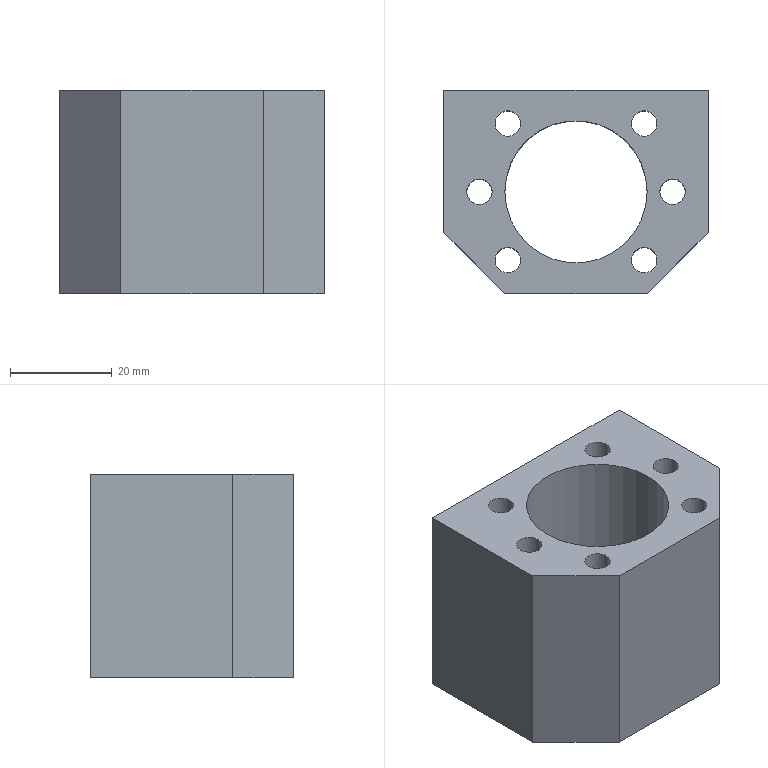Part | SolidWorks | features BaseBody 1 | 1 solid | 34 faces | box 52 x 40 x 40 mm | volume 47312 mm3 | cylinder 22 | plane 12 | commonest cylinder face diameters 5 x20 28 x2
STEP:
#1=CARTESIAN_POINT('',(-17.5,10.,8.));
#2=VERTEX_POINT('',#1);
#3=CARTESIAN_POINT('',(-22.5,10.,8.));
#4=VERTEX_POINT('',#3);
#5=CARTESIAN_POINT('',(-20.,10.,8.));
#6=DIRECTION('',(0.,1.,0.));
#7=DIRECTION('',(-1.,0.,0.));
#8=AXIS2_PLACEMENT_3D('',#5,#6,#7);
#9=CIRCLE('',#8,2.5);
#10=EDGE_CURVE('',#2,#4,#9,.T.);
#11=ORIENTED_EDGE('',*,*,#10,.F.);
#12=CARTESIAN_POINT('',(-17.5,20.,8.));
#13=VERTEX_POINT('',#12);
#14=CARTESIAN_POINT('',(-17.5,10.,8.));
#15=DIRECTION('',(0.,1.,0.));
#16=VECTOR('',#15,1000.);
#17=LINE('',#14,#16);
#18=EDGE_CURVE('',#2,#13,#17,.T.);
#19=ORIENTED_EDGE('',*,*,#18,.T.);
#20=CARTESIAN_POINT('',(-22.5,20.,8.));
#21=VERTEX_POINT('',#20);
#22=CARTESIAN_POINT('',(-20.,20.,8.));
#23=DIRECTION('',(0.,1.,0.));
#24=DIRECTION('',(-1.,0.,0.));
#25=AXIS2_PLACEMENT_3D('',#22,#23,#24);
#26=CIRCLE('',#25,2.5);
#27=EDGE_CURVE('',#13,#21,#26,.T.);
#28=ORIENTED_EDGE('',*,*,#27,.T.);
#29=CARTESIAN_POINT('',(-22.5,10.,8.));
#30=DIRECTION('',(0.,1.,0.));
#31=VECTOR('',#30,1000.);
#32=LINE('',#29,#31);
#33=EDGE_CURVE('',#4,#21,#32,.T.);
#34=ORIENTED_EDGE('',*,*,#33,.F.);
#35=EDGE_LOOP('',(#11,#19,#28,#34));
#36=FACE_OUTER_BOUND('',#35,.T.);
#37=CARTESIAN_POINT('',(-20.,10.,8.));
#38=DIRECTION('',(0.,1.,0.));
#39=DIRECTION('',(-1.,0.,0.));
#40=AXIS2_PLACEMENT_3D('',#37,#38,#39);
#41=CYLINDRICAL_SURFACE('',#40,2.5);
#42=ADVANCED_FACE('',(#36),#41,.F.);
#43=CARTESIAN_POINT('',(-17.5,10.,32.));
#44=VERTEX_POINT('',#43);
#45=CARTESIAN_POINT('',(-22.5,10.,32.));
#46=VERTEX_POINT('',#45);
#47=CARTESIAN_POINT('',(-20.,10.,32.));
#48=DIRECTION('',(0.,1.,0.));
#49=DIRECTION('',(-1.,0.,0.));
#50=AXIS2_PLACEMENT_3D('',#47,#48,#49);
#51=CIRCLE('',#50,2.5);
#52=EDGE_CURVE('',#44,#46,#51,.T.);
#53=ORIENTED_EDGE('',*,*,#52,.F.);
#54=CARTESIAN_POINT('',(-17.5,20.,32.));
#55=VERTEX_POINT('',#54);
#56=CARTESIAN_POINT('',(-17.5,10.,32.));
#57=DIRECTION('',(0.,1.,0.));
#58=VECTOR('',#57,1000.);
#59=LINE('',#56,#58);
#60=EDGE_CURVE('',#44,#55,#59,.T.);
#61=ORIENTED_EDGE('',*,*,#60,.T.);
#62=CARTESIAN_POINT('',(-22.5,20.,32.));
#63=VERTEX_POINT('',#62);
#64=CARTESIAN_POINT('',(-20.,20.,32.));
#65=DIRECTION('',(0.,1.,0.));
#66=DIRECTION('',(-1.,0.,0.));
#67=AXIS2_PLACEMENT_3D('',#64,#65,#66);
#68=CIRCLE('',#67,2.5);
#69=EDGE_CURVE('',#55,#63,#68,.T.);
#70=ORIENTED_EDGE('',*,*,#69,.T.);
#71=CARTESIAN_POINT('',(-22.5,10.,32.));
#72=DIRECTION('',(0.,1.,0.));
#73=VECTOR('',#72,1000.);
#74=LINE('',#71,#73);
#75=EDGE_CURVE('',#46,#63,#74,.T.);
#76=ORIENTED_EDGE('',*,*,#75,.F.);
#77=EDGE_LOOP('',(#53,#61,#70,#76));
#78=FACE_OUTER_BOUND('',#77,.T.);
#79=CARTESIAN_POINT('',(-20.,10.,32.));
#80=DIRECTION('',(0.,1.,0.));
#81=DIRECTION('',(-1.,0.,0.));
#82=AXIS2_PLACEMENT_3D('',#79,#80,#81);
#83=CYLINDRICAL_SURFACE('',#82,2.5);
#84=ADVANCED_FACE('',(#78),#83,.F.);
#85=CARTESIAN_POINT('',(22.5,10.,32.));
#86=VERTEX_POINT('',#85);
#87=CARTESIAN_POINT('',(17.5,10.,32.));
#88=VERTEX_POINT('',#87);
#89=CARTESIAN_POINT('',(20.,10.,32.));
#90=DIRECTION('',(0.,1.,0.));
#91=DIRECTION('',(-1.,0.,0.));
#92=AXIS2_PLACEMENT_3D('',#89,#90,#91);
#93=CIRCLE('',#92,2.5);
#94=EDGE_CURVE('',#86,#88,#93,.T.);
#95=ORIENTED_EDGE('',*,*,#94,.F.);
#96=CARTESIAN_POINT('',(22.5,20.,32.));
#97=VERTEX_POINT('',#96);
#98=CARTESIAN_POINT('',(22.5,10.,32.));
#99=DIRECTION('',(0.,1.,0.));
#100=VECTOR('',#99,1000.);
#101=LINE('',#98,#100);
#102=EDGE_CURVE('',#86,#97,#101,.T.);
#103=ORIENTED_EDGE('',*,*,#102,.T.);
#104=CARTESIAN_POINT('',(17.5,20.,32.));
#105=VERTEX_POINT('',#104);
#106=CARTESIAN_POINT('',(20.,20.,32.));
#107=DIRECTION('',(0.,1.,0.));
#108=DIRECTION('',(-1.,0.,0.));
#109=AXIS2_PLACEMENT_3D('',#106,#107,#108);
#110=CIRCLE('',#109,2.5);
#111=EDGE_CURVE('',#97,#105,#110,.T.);
#112=ORIENTED_EDGE('',*,*,#111,.T.);
#113=CARTESIAN_POINT('',(17.5,10.,32.));
#114=DIRECTION('',(0.,1.,0.));
#115=VECTOR('',#114,1000.);
#116=LINE('',#113,#115);
#117=EDGE_CURVE('',#88,#105,#116,.T.);
#118=ORIENTED_EDGE('',*,*,#117,.F.);
#119=EDGE_LOOP('',(#95,#103,#112,#118));
#120=FACE_OUTER_BOUND('',#119,.T.);
#121=CARTESIAN_POINT('',(20.,10.,32.));
#122=DIRECTION('',(0.,1.,0.));
#123=DIRECTION('',(-1.,0.,0.));
#124=AXIS2_PLACEMENT_3D('',#121,#122,#123);
#125=CYLINDRICAL_SURFACE('',#124,2.5);
#126=ADVANCED_FACE('',(#120),#125,.F.);
#127=CARTESIAN_POINT('',(22.5,10.,8.));
#128=VERTEX_POINT('',#127);
#129=CARTESIAN_POINT('',(17.5,10.,8.));
#130=VERTEX_POINT('',#129);
#131=CARTESIAN_POINT('',(20.,10.,8.));
#132=DIRECTION('',(0.,1.,0.));
#133=DIRECTION('',(-1.,0.,0.));
#134=AXIS2_PLACEMENT_3D('',#131,#132,#133);
#135=CIRCLE('',#134,2.5);
#136=EDGE_CURVE('',#128,#130,#135,.T.);
#137=ORIENTED_EDGE('',*,*,#136,.F.);
#138=CARTESIAN_POINT('',(22.5,20.,8.));
#139=VERTEX_POINT('',#138);
#140=CARTESIAN_POINT('',(22.5,10.,8.));
#141=DIRECTION('',(0.,1.,0.));
#142=VECTOR('',#141,1000.);
#143=LINE('',#140,#142);
#144=EDGE_CURVE('',#128,#139,#143,.T.);
#145=ORIENTED_EDGE('',*,*,#144,.T.);
#146=CARTESIAN_POINT('',(17.5,20.,8.));
#147=VERTEX_POINT('',#146);
#148=CARTESIAN_POINT('',(20.,20.,8.));
#149=DIRECTION('',(0.,1.,0.));
#150=DIRECTION('',(-1.,0.,0.));
#151=AXIS2_PLACEMENT_3D('',#148,#149,#150);
#152=CIRCLE('',#151,2.5);
#153=EDGE_CURVE('',#139,#147,#152,.T.);
#154=ORIENTED_EDGE('',*,*,#153,.T.);
#155=CARTESIAN_POINT('',(17.5,10.,8.));
#156=DIRECTION('',(0.,1.,0.));
#157=VECTOR('',#156,1000.);
#158=LINE('',#155,#157);
#159=EDGE_CURVE('',#130,#147,#158,.T.);
#160=ORIENTED_EDGE('',*,*,#159,.F.);
#161=EDGE_LOOP('',(#137,#145,#154,#160));
#162=FACE_OUTER_BOUND('',#161,.T.);
#163=CARTESIAN_POINT('',(20.,10.,8.));
#164=DIRECTION('',(0.,1.,0.));
#165=DIRECTION('',(-1.,0.,0.));
#166=AXIS2_PLACEMENT_3D('',#163,#164,#165);
#167=CYLINDRICAL_SURFACE('',#166,2.5);
#168=ADVANCED_FACE('',(#162),#167,.F.);
#169=CARTESIAN_POINT('',(21.5,0.,40.));
#170=VERTEX_POINT('',#169);
#171=CARTESIAN_POINT('',(16.5,0.,40.));
#172=VERTEX_POINT('',#171);
#173=CARTESIAN_POINT('',(19.,0.,40.));
#174=DIRECTION('',(0.,0.,-1.));
#175=DIRECTION('',(-1.,0.,0.));
#176=AXIS2_PLACEMENT_3D('',#173,#174,#175);
#177=CIRCLE('',#176,2.5);
#178=EDGE_CURVE('',#170,#172,#177,.T.);
#179=ORIENTED_EDGE('',*,*,#178,.F.);
#180=CARTESIAN_POINT('',(21.5,0.,0.));
#181=VERTEX_POINT('',#180);
#182=CARTESIAN_POINT('',(21.5,0.,40.));
#183=DIRECTION('',(0.,0.,-1.));
#184=VECTOR('',#183,1000.);
#185=LINE('',#182,#184);
#186=EDGE_CURVE('',#170,#181,#185,.T.);
#187=ORIENTED_EDGE('',*,*,#186,.T.);
#188=CARTESIAN_POINT('',(16.5,0.,0.));
#189=VERTEX_POINT('',#188);
#190=CARTESIAN_POINT('',(19.,0.,0.));
#191=DIRECTION('',(0.,0.,-1.));
#192=DIRECTION('',(-1.,0.,0.));
#193=AXIS2_PLACEMENT_3D('',#190,#191,#192);
#194=CIRCLE('',#193,2.5);
#195=EDGE_CURVE('',#181,#189,#194,.T.);
#196=ORIENTED_EDGE('',*,*,#195,.T.);
#197=CARTESIAN_POINT('',(16.5,0.,40.));
#198=DIRECTION('',(0.,0.,-1.));
#199=VECTOR('',#198,1000.);
#200=LINE('',#197,#199);
#201=EDGE_CURVE('',#172,#189,#200,.T.);
#202=ORIENTED_EDGE('',*,*,#201,.F.);
#203=EDGE_LOOP('',(#179,#187,#196,#202));
#204=FACE_OUTER_BOUND('',#203,.T.);
#205=CARTESIAN_POINT('',(19.,0.,40.));
#206=DIRECTION('',(0.,0.,-1.));
#207=DIRECTION('',(-1.,0.,0.));
#208=AXIS2_PLACEMENT_3D('',#205,#206,#207);
#209=CYLINDRICAL_SURFACE('',#208,2.5);
#210=ADVANCED_FACE('',(#204),#209,.F.);
#211=CARTESIAN_POINT('',(15.935,13.435,40.));
#212=VERTEX_POINT('',#211);
#213=CARTESIAN_POINT('',(10.935,13.435,40.));
#214=VERTEX_POINT('',#213);
#215=CARTESIAN_POINT('',(13.435,13.435,40.));
#216=DIRECTION('',(0.,0.,-1.));
#217=DIRECTION('',(-1.,0.,0.));
#218=AXIS2_PLACEMENT_3D('',#215,#216,#217);
#219=CIRCLE('',#218,2.5);
#220=EDGE_CURVE('',#212,#214,#219,.T.);
#221=ORIENTED_EDGE('',*,*,#220,.F.);
#222=CARTESIAN_POINT('',(15.935,13.435,0.));
#223=VERTEX_POINT('',#222);
#224=CARTESIAN_POINT('',(15.935,13.435,40.));
#225=DIRECTION('',(0.,0.,-1.));
#226=VECTOR('',#225,1000.);
#227=LINE('',#224,#226);
#228=EDGE_CURVE('',#212,#223,#227,.T.);
#229=ORIENTED_EDGE('',*,*,#228,.T.);
#230=CARTESIAN_POINT('',(10.935,13.435,0.));
#231=VERTEX_POINT('',#230);
#232=CARTESIAN_POINT('',(13.435,13.435,0.));
#233=DIRECTION('',(0.,0.,-1.));
#234=DIRECTION('',(-1.,0.,0.));
#235=AXIS2_PLACEMENT_3D('',#232,#233,#234);
#236=CIRCLE('',#235,2.5);
#237=EDGE_CURVE('',#223,#231,#236,.T.);
#238=ORIENTED_EDGE('',*,*,#237,.T.);
#239=CARTESIAN_POINT('',(10.935,13.435,40.));
#240=DIRECTION('',(0.,0.,-1.));
#241=VECTOR('',#240,1000.);
#242=LINE('',#239,#241);
#243=EDGE_CURVE('',#214,#231,#242,.T.);
#244=ORIENTED_EDGE('',*,*,#243,.F.);
#245=EDGE_LOOP('',(#221,#229,#238,#244));
#246=FACE_OUTER_BOUND('',#245,.T.);
#247=CARTESIAN_POINT('',(13.435,13.435,40.));
#248=DIRECTION('',(0.,0.,-1.));
#249=DIRECTION('',(-1.,0.,0.));
#250=AXIS2_PLACEMENT_3D('',#247,#248,#249);
#251=CYLINDRICAL_SURFACE('',#250,2.5);
#252=ADVANCED_FACE('',(#246),#251,.F.);
#253=CARTESIAN_POINT('',(15.935,-13.435,40.));
#254=VERTEX_POINT('',#253);
#255=CARTESIAN_POINT('',(10.935,-13.435,40.));
#256=VERTEX_POINT('',#255);
#257=CARTESIAN_POINT('',(13.435,-13.435,40.));
#258=DIRECTION('',(0.,0.,-1.));
#259=DIRECTION('',(-1.,0.,0.));
#260=AXIS2_PLACEMENT_3D('',#257,#258,#259);
#261=CIRCLE('',#260,2.5);
#262=EDGE_CURVE('',#254,#256,#261,.T.);
#263=ORIENTED_EDGE('',*,*,#262,.F.);
#264=CARTESIAN_POINT('',(15.935,-13.435,0.));
#265=VERTEX_POINT('',#264);
#266=CARTESIAN_POINT('',(15.935,-13.435,40.));
#267=DIRECTION('',(0.,0.,-1.));
#268=VECTOR('',#267,1000.);
#269=LINE('',#266,#268);
#270=EDGE_CURVE('',#254,#265,#269,.T.);
#271=ORIENTED_EDGE('',*,*,#270,.T.);
#272=CARTESIAN_POINT('',(10.935,-13.435,0.));
#273=VERTEX_POINT('',#272);
#274=CARTESIAN_POINT('',(13.435,-13.435,0.));
#275=DIRECTION('',(0.,0.,-1.));
#276=DIRECTION('',(-1.,0.,0.));
#277=AXIS2_PLACEMENT_3D('',#274,#275,#276);
#278=CIRCLE('',#277,2.5);
#279=EDGE_CURVE('',#265,#273,#278,.T.);
#280=ORIENTED_EDGE('',*,*,#279,.T.);
#281=CARTESIAN_POINT('',(10.935,-13.435,40.));
#282=DIRECTION('',(0.,0.,-1.));
#283=VECTOR('',#282,1000.);
#284=LINE('',#281,#283);
#285=EDGE_CURVE('',#256,#273,#284,.T.);
#286=ORIENTED_EDGE('',*,*,#285,.F.);
#287=EDGE_LOOP('',(#263,#271,#280,#286));
#288=FACE_OUTER_BOUND('',#287,.T.);
#289=CARTESIAN_POINT('',(13.435,-13.435,40.));
#290=DIRECTION('',(0.,0.,-1.));
#291=DIRECTION('',(-1.,0.,0.));
#292=AXIS2_PLACEMENT_3D('',#289,#290,#291);
#293=CYLINDRICAL_SURFACE('',#292,2.5);
#294=ADVANCED_FACE('',(#288),#293,.F.);
#295=CARTESIAN_POINT('',(-10.935,-13.435,40.));
#296=VERTEX_POINT('',#295);
#297=CARTESIAN_POINT('',(-15.935,-13.435,40.));
#298=VERTEX_POINT('',#297);
#299=CARTESIAN_POINT('',(-13.435,-13.435,40.));
#300=DIRECTION('',(0.,0.,-1.));
#301=DIRECTION('',(-1.,0.,0.));
#302=AXIS2_PLACEMENT_3D('',#299,#300,#301);
#303=CIRCLE('',#302,2.5);
#304=EDGE_CURVE('',#296,#298,#303,.T.);
#305=ORIENTED_EDGE('',*,*,#304,.F.);
#306=CARTESIAN_POINT('',(-10.935,-13.435,0.));
#307=VERTEX_POINT('',#306);
#308=CARTESIAN_POINT('',(-10.935,-13.435,40.));
#309=DIRECTION('',(0.,0.,-1.));
#310=VECTOR('',#309,1000.);
#311=LINE('',#308,#310);
#312=EDGE_CURVE('',#296,#307,#311,.T.);
#313=ORIENTED_EDGE('',*,*,#312,.T.);
#314=CARTESIAN_POINT('',(-15.935,-13.435,0.));
#315=VERTEX_POINT('',#314);
#316=CARTESIAN_POINT('',(-13.435,-13.435,0.));
#317=DIRECTION('',(0.,0.,-1.));
#318=DIRECTION('',(-1.,0.,0.));
#319=AXIS2_PLACEMENT_3D('',#316,#317,#318);
#320=CIRCLE('',#319,2.5);
#321=EDGE_CURVE('',#307,#315,#320,.T.);
#322=ORIENTED_EDGE('',*,*,#321,.T.);
#323=CARTESIAN_POINT('',(-15.935,-13.435,40.));
#324=DIRECTION('',(0.,0.,-1.));
#325=VECTOR('',#324,1000.);
#326=LINE('',#323,#325);
#327=EDGE_CURVE('',#298,#315,#326,.T.);
#328=ORIENTED_EDGE('',*,*,#327,.F.);
#329=EDGE_LOOP('',(#305,#313,#322,#328));
#330=FACE_OUTER_BOUND('',#329,.T.);
#331=CARTESIAN_POINT('',(-13.435,-13.435,40.));
#332=DIRECTION('',(0.,0.,-1.));
#333=DIRECTION('',(-1.,0.,0.));
#334=AXIS2_PLACEMENT_3D('',#331,#332,#333);
#335=CYLINDRICAL_SURFACE('',#334,2.5);
#336=ADVANCED_FACE('',(#330),#335,.F.);
#337=CARTESIAN_POINT('',(-10.935,13.435,40.));
#338=VERTEX_POINT('',#337);
#339=CARTESIAN_POINT('',(-15.935,13.435,40.));
#340=VERTEX_POINT('',#339);
#341=CARTESIAN_POINT('',(-13.435,13.435,40.));
#342=DIRECTION('',(0.,0.,-1.));
#343=DIRECTION('',(-1.,0.,0.));
#344=AXIS2_PLACEMENT_3D('',#341,#342,#343);
#345=CIRCLE('',#344,2.5);
#346=EDGE_CURVE('',#338,#340,#345,.T.);
#347=ORIENTED_EDGE('',*,*,#346,.F.);
#348=CARTESIAN_POINT('',(-10.935,13.435,0.));
#349=VERTEX_POINT('',#348);
#350=CARTESIAN_POINT('',(-10.935,13.435,40.));
#351=DIRECTION('',(0.,0.,-1.));
#352=VECTOR('',#351,1000.);
#353=LINE('',#350,#352);
#354=EDGE_CURVE('',#338,#349,#353,.T.);
#355=ORIENTED_EDGE('',*,*,#354,.T.);
#356=CARTESIAN_POINT('',(-15.935,13.435,0.));
#357=VERTEX_POINT('',#356);
#358=CARTESIAN_POINT('',(-13.435,13.435,0.));
#359=DIRECTION('',(0.,0.,-1.));
#360=DIRECTION('',(-1.,0.,0.));
#361=AXIS2_PLACEMENT_3D('',#358,#359,#360);
#362=CIRCLE('',#361,2.5);
#363=EDGE_CURVE('',#349,#357,#362,.T.);
#364=ORIENTED_EDGE('',*,*,#363,.T.);
#365=CARTESIAN_POINT('',(-15.935,13.435,40.));
#366=DIRECTION('',(0.,0.,-1.));
#367=VECTOR('',#366,1000.);
#368=LINE('',#365,#367);
#369=EDGE_CURVE('',#340,#357,#368,.T.);
#370=ORIENTED_EDGE('',*,*,#369,.F.);
#371=EDGE_LOOP('',(#347,#355,#364,#370));
#372=FACE_OUTER_BOUND('',#371,.T.);
#373=CARTESIAN_POINT('',(-13.435,13.435,40.));
#374=DIRECTION('',(0.,0.,-1.));
#375=DIRECTION('',(-1.,0.,0.));
#376=AXIS2_PLACEMENT_3D('',#373,#374,#375);
#377=CYLINDRICAL_SURFACE('',#376,2.5);
#378=ADVANCED_FACE('',(#372),#377,.F.);
#379=CARTESIAN_POINT('',(-16.5,0.,40.));
#380=VERTEX_POINT('',#379);
#381=CARTESIAN_POINT('',(-21.5,0.,40.));
#382=VERTEX_POINT('',#381);
#383=CARTESIAN_POINT('',(-19.,0.,40.));
#384=DIRECTION('',(0.,0.,-1.));
#385=DIRECTION('',(-1.,0.,0.));
#386=AXIS2_PLACEMENT_3D('',#383,#384,#385);
#387=CIRCLE('',#386,2.5);
#388=EDGE_CURVE('',#380,#382,#387,.T.);
#389=ORIENTED_EDGE('',*,*,#388,.F.);
#390=CARTESIAN_POINT('',(-16.5,0.,0.));
#391=VERTEX_POINT('',#390);
#392=CARTESIAN_POINT('',(-16.5,0.,40.));
#393=DIRECTION('',(0.,0.,-1.));
#394=VECTOR('',#393,1000.);
#395=LINE('',#392,#394);
#396=EDGE_CURVE('',#380,#391,#395,.T.);
#397=ORIENTED_EDGE('',*,*,#396,.T.);
#398=CARTESIAN_POINT('',(-21.5,0.,0.));
#399=VERTEX_POINT('',#398);
#400=CARTESIAN_POINT('',(-19.,0.,0.));
#401=DIRECTION('',(0.,0.,-1.));
#402=DIRECTION('',(-1.,0.,0.));
#403=AXIS2_PLACEMENT_3D('',#400,#401,#402);
#404=CIRCLE('',#403,2.5);
#405=EDGE_CURVE('',#391,#399,#404,.T.);
#406=ORIENTED_EDGE('',*,*,#405,.T.);
#407=CARTESIAN_POINT('',(-21.5,0.,40.));
#408=DIRECTION('',(0.,0.,-1.));
#409=VECTOR('',#408,1000.);
#410=LINE('',#407,#409);
#411=EDGE_CURVE('',#382,#399,#410,.T.);
#412=ORIENTED_EDGE('',*,*,#411,.F.);
#413=EDGE_LOOP('',(#389,#397,#406,#412));
#414=FACE_OUTER_BOUND('',#413,.T.);
#415=CARTESIAN_POINT('',(-19.,0.,40.));
#416=DIRECTION('',(0.,0.,-1.));
#417=DIRECTION('',(-1.,0.,0.));
#418=AXIS2_PLACEMENT_3D('',#415,#416,#417);
#419=CYLINDRICAL_SURFACE('',#418,2.5);
#420=ADVANCED_FACE('',(#414),#419,.F.);
#421=CARTESIAN_POINT('',(14.,0.,40.));
#422=VERTEX_POINT('',#421);
#423=CARTESIAN_POINT('',(-14.,0.,40.));
#424=VERTEX_POINT('',#423);
#425=CARTESIAN_POINT('',(0.,0.,40.));
#426=DIRECTION('',(0.,0.,-1.));
#427=DIRECTION('',(-1.,0.,0.));
#428=AXIS2_PLACEMENT_3D('',#425,#426,#427);
#429=CIRCLE('',#428,14.);
#430=EDGE_CURVE('',#422,#424,#429,.T.);
#431=ORIENTED_EDGE('',*,*,#430,.F.);
#432=CARTESIAN_POINT('',(14.,0.,0.));
#433=VERTEX_POINT('',#432);
#434=CARTESIAN_POINT('',(14.,0.,40.));
#435=DIRECTION('',(0.,0.,-1.));
#436=VECTOR('',#435,1000.);
#437=LINE('',#434,#436);
#438=EDGE_CURVE('',#422,#433,#437,.T.);
#439=ORIENTED_EDGE('',*,*,#438,.T.);
#440=CARTESIAN_POINT('',(-14.,0.,0.));
#441=VERTEX_POINT('',#440);
#442=CARTESIAN_POINT('',(0.,0.,0.));
#443=DIRECTION('',(0.,0.,-1.));
#444=DIRECTION('',(-1.,0.,0.));
#445=AXIS2_PLACEMENT_3D('',#442,#443,#444);
#446=CIRCLE('',#445,14.);
#447=EDGE_CURVE('',#433,#441,#446,.T.);
#448=ORIENTED_EDGE('',*,*,#447,.T.);
#449=CARTESIAN_POINT('',(-14.,0.,40.));
#450=DIRECTION('',(0.,0.,-1.));
#451=VECTOR('',#450,1000.);
#452=LINE('',#449,#451);
#453=EDGE_CURVE('',#424,#441,#452,.T.);
#454=ORIENTED_EDGE('',*,*,#453,.F.);
#455=EDGE_LOOP('',(#431,#439,#448,#454));
#456=FACE_OUTER_BOUND('',#455,.T.);
#457=CARTESIAN_POINT('',(0.,0.,40.));
#458=DIRECTION('',(0.,0.,-1.));
#459=DIRECTION('',(-1.,0.,0.));
#460=AXIS2_PLACEMENT_3D('',#457,#458,#459);
#461=CYLINDRICAL_SURFACE('',#460,14.);
#462=ADVANCED_FACE('',(#456),#461,.F.);
#463=CARTESIAN_POINT('',(-26.,20.,40.));
#464=VERTEX_POINT('',#463);
#465=CARTESIAN_POINT('',(-26.,20.,0.));
#466=VERTEX_POINT('',#465);
#467=CARTESIAN_POINT('',(-26.,20.,40.));
#468=DIRECTION('',(0.,0.,-1.));
#469=VECTOR('',#468,1000.);
#470=LINE('',#467,#469);
#471=EDGE_CURVE('',#464,#466,#470,.T.);
#472=ORIENTED_EDGE('',*,*,#471,.F.);
#473=CARTESIAN_POINT('',(26.,20.,40.));
#474=VERTEX_POINT('',#473);
#475=CARTESIAN_POINT('',(26.,20.,40.));
#476=DIRECTION('',(-1.,0.,0.));
#477=VECTOR('',#476,1000.);
#478=LINE('',#475,#477);
#479=EDGE_CURVE('',#474,#464,#478,.T.);
#480=ORIENTED_EDGE('',*,*,#479,.F.);
#481=CARTESIAN_POINT('',(26.,20.,0.));
#482=VERTEX_POINT('',#481);
#483=CARTESIAN_POINT('',(26.,20.,40.));
#484=DIRECTION('',(0.,0.,1.));
#485=VECTOR('',#484,1000.);
#486=LINE('',#483,#485);
#487=EDGE_CURVE('',#482,#474,#486,.T.);
#488=ORIENTED_EDGE('',*,*,#487,.F.);
#489=CARTESIAN_POINT('',(26.,20.,0.));
#490=DIRECTION('',(1.,0.,0.));
#491=VECTOR('',#490,1000.);
#492=LINE('',#489,#491);
#493=EDGE_CURVE('',#466,#482,#492,.T.);
#494=ORIENTED_EDGE('',*,*,#493,.F.);
#495=EDGE_LOOP('',(#472,#480,#488,#494));
#496=FACE_OUTER_BOUND('',#495,.T.);
#497=CARTESIAN_POINT('',(-20.,20.,8.));
#498=DIRECTION('',(0.,1.,0.));
#499=DIRECTION('',(-1.,0.,0.));
#500=AXIS2_PLACEMENT_3D('',#497,#498,#499);
#501=CIRCLE('',#500,2.5);
#502=EDGE_CURVE('',#21,#13,#501,.T.);
#503=ORIENTED_EDGE('',*,*,#502,.F.);
#504=ORIENTED_EDGE('',*,*,#27,.F.);
#505=EDGE_LOOP('',(#503,#504));
#506=FACE_BOUND('',#505,.T.);
#507=CARTESIAN_POINT('',(-20.,20.,32.));
#508=DIRECTION('',(0.,1.,0.));
#509=DIRECTION('',(-1.,0.,0.));
#510=AXIS2_PLACEMENT_3D('',#507,#508,#509);
#511=CIRCLE('',#510,2.5);
#512=EDGE_CURVE('',#63,#55,#511,.T.);
#513=ORIENTED_EDGE('',*,*,#512,.F.);
#514=ORIENTED_EDGE('',*,*,#69,.F.);
#515=EDGE_LOOP('',(#513,#514));
#516=FACE_BOUND('',#515,.T.);
#517=CARTESIAN_POINT('',(20.,20.,32.));
#518=DIRECTION('',(0.,1.,0.));
#519=DIRECTION('',(-1.,0.,0.));
#520=AXIS2_PLACEMENT_3D('',#517,#518,#519);
#521=CIRCLE('',#520,2.5);
#522=EDGE_CURVE('',#105,#97,#521,.T.);
#523=ORIENTED_EDGE('',*,*,#522,.F.);
#524=ORIENTED_EDGE('',*,*,#111,.F.);
#525=EDGE_LOOP('',(#523,#524));
#526=FACE_BOUND('',#525,.T.);
#527=CARTESIAN_POINT('',(20.,20.,8.));
#528=DIRECTION('',(0.,1.,0.));
#529=DIRECTION('',(-1.,0.,0.));
#530=AXIS2_PLACEMENT_3D('',#527,#528,#529);
#531=CIRCLE('',#530,2.5);
#532=EDGE_CURVE('',#147,#139,#531,.T.);
#533=ORIENTED_EDGE('',*,*,#532,.F.);
#534=ORIENTED_EDGE('',*,*,#153,.F.);
#535=EDGE_LOOP('',(#533,#534));
#536=FACE_BOUND('',#535,.T.);
#537=CARTESIAN_POINT('',(26.,20.,40.));
#538=DIRECTION('',(0.,-1.,0.));
#539=DIRECTION('',(1.,0.,0.));
#540=AXIS2_PLACEMENT_3D('',#537,#538,#539);
#541=PLANE('',#540);
#542=ADVANCED_FACE('',(#496,#506,#516,#526,#536),#541,.F.);
#543=CARTESIAN_POINT('',(19.,0.,0.));
#544=DIRECTION('',(0.,0.,-1.));
#545=DIRECTION('',(-1.,0.,0.));
#546=AXIS2_PLACEMENT_3D('',#543,#544,#545);
#547=CIRCLE('',#546,2.5);
#548=EDGE_CURVE('',#189,#181,#547,.T.);
#549=ORIENTED_EDGE('',*,*,#548,.F.);
#550=ORIENTED_EDGE('',*,*,#195,.F.);
#551=EDGE_LOOP('',(#549,#550));
#552=FACE_BOUND('',#551,.T.);
#553=CARTESIAN_POINT('',(13.435,13.435,0.));
#554=DIRECTION('',(0.,0.,-1.));
#555=DIRECTION('',(-1.,0.,0.));
#556=AXIS2_PLACEMENT_3D('',#553,#554,#555);
#557=CIRCLE('',#556,2.5);
#558=EDGE_CURVE('',#231,#223,#557,.T.);
#559=ORIENTED_EDGE('',*,*,#558,.F.);
#560=ORIENTED_EDGE('',*,*,#237,.F.);
#561=EDGE_LOOP('',(#559,#560));
#562=FACE_BOUND('',#561,.T.);
#563=CARTESIAN_POINT('',(13.435,-13.435,0.));
#564=DIRECTION('',(0.,0.,-1.));
#565=DIRECTION('',(-1.,0.,0.));
#566=AXIS2_PLACEMENT_3D('',#563,#564,#565);
#567=CIRCLE('',#566,2.5);
#568=EDGE_CURVE('',#273,#265,#567,.T.);
#569=ORIENTED_EDGE('',*,*,#568,.F.);
#570=ORIENTED_EDGE('',*,*,#279,.F.);
#571=EDGE_LOOP('',(#569,#570));
#572=FACE_BOUND('',#571,.T.);
#573=CARTESIAN_POINT('',(-13.435,-13.435,0.));
#574=DIRECTION('',(0.,0.,-1.));
#575=DIRECTION('',(-1.,0.,0.));
#576=AXIS2_PLACEMENT_3D('',#573,#574,#575);
#577=CIRCLE('',#576,2.5);
#578=EDGE_CURVE('',#315,#307,#577,.T.);
#579=ORIENTED_EDGE('',*,*,#578,.F.);
#580=ORIENTED_EDGE('',*,*,#321,.F.);
#581=EDGE_LOOP('',(#579,#580));
#582=FACE_BOUND('',#581,.T.);
#583=CARTESIAN_POINT('',(-13.435,13.435,0.));
#584=DIRECTION('',(0.,0.,-1.));
#585=DIRECTION('',(-1.,0.,0.));
#586=AXIS2_PLACEMENT_3D('',#583,#584,#585);
#587=CIRCLE('',#586,2.5);
#588=EDGE_CURVE('',#357,#349,#587,.T.);
#589=ORIENTED_EDGE('',*,*,#588,.F.);
#590=ORIENTED_EDGE('',*,*,#363,.F.);
#591=EDGE_LOOP('',(#589,#590));
#592=FACE_BOUND('',#591,.T.);
#593=CARTESIAN_POINT('',(-19.,0.,0.));
#594=DIRECTION('',(0.,0.,-1.));
#595=DIRECTION('',(-1.,0.,0.));
#596=AXIS2_PLACEMENT_3D('',#593,#594,#595);
#597=CIRCLE('',#596,2.5);
#598=EDGE_CURVE('',#399,#391,#597,.T.);
#599=ORIENTED_EDGE('',*,*,#598,.F.);
#600=ORIENTED_EDGE('',*,*,#405,.F.);
#601=EDGE_LOOP('',(#599,#600));
#602=FACE_BOUND('',#601,.T.);
#603=CARTESIAN_POINT('',(0.,0.,0.));
#604=DIRECTION('',(0.,0.,-1.));
#605=DIRECTION('',(-1.,0.,0.));
#606=AXIS2_PLACEMENT_3D('',#603,#604,#605);
#607=CIRCLE('',#606,14.);
#608=EDGE_CURVE('',#441,#433,#607,.T.);
#609=ORIENTED_EDGE('',*,*,#608,.F.);
#610=ORIENTED_EDGE('',*,*,#447,.F.);
#611=EDGE_LOOP('',(#609,#610));
#612=FACE_BOUND('',#611,.T.);
#613=ORIENTED_EDGE('',*,*,#493,.T.);
#614=CARTESIAN_POINT('',(26.,-8.,0.));
#615=VERTEX_POINT('',#614);
#616=CARTESIAN_POINT('',(26.,0.,0.));
#617=DIRECTION('',(0.,1.,0.));
#618=VECTOR('',#617,1000.);
#619=LINE('',#616,#618);
#620=EDGE_CURVE('',#615,#482,#619,.T.);
#621=ORIENTED_EDGE('',*,*,#620,.F.);
#622=CARTESIAN_POINT('',(14.,-20.,0.));
#623=VERTEX_POINT('',#622);
#624=CARTESIAN_POINT('',(14.,-20.,0.));
#625=DIRECTION('',(0.7071,0.7071,0.));
#626=VECTOR('',#625,1000.);
#627=LINE('',#624,#626);
#628=EDGE_CURVE('',#623,#615,#627,.T.);
#629=ORIENTED_EDGE('',*,*,#628,.F.);
#630=CARTESIAN_POINT('',(-14.,-20.,0.));
#631=VERTEX_POINT('',#630);
#632=CARTESIAN_POINT('',(0.,-20.,0.));
#633=DIRECTION('',(1.,0.,0.));
#634=VECTOR('',#633,1000.);
#635=LINE('',#632,#634);
#636=EDGE_CURVE('',#631,#623,#635,.T.);
#637=ORIENTED_EDGE('',*,*,#636,.F.);
#638=CARTESIAN_POINT('',(-26.,-8.,0.));
#639=VERTEX_POINT('',#638);
#640=CARTESIAN_POINT('',(-26.,-8.,0.));
#641=DIRECTION('',(0.7071,-0.7071,0.));
#642=VECTOR('',#641,1000.);
#643=LINE('',#640,#642);
#644=EDGE_CURVE('',#639,#631,#643,.T.);
#645=ORIENTED_EDGE('',*,*,#644,.F.);
#646=CARTESIAN_POINT('',(-26.,0.,0.));
#647=DIRECTION('',(0.,-1.,0.));
#648=VECTOR('',#647,1000.);
#649=LINE('',#646,#648);
#650=EDGE_CURVE('',#466,#639,#649,.T.);
#651=ORIENTED_EDGE('',*,*,#650,.F.);
#652=EDGE_LOOP('',(#613,#621,#629,#637,#645,#651));
#653=FACE_OUTER_BOUND('',#652,.T.);
#654=CARTESIAN_POINT('',(0.,0.,0.));
#655=DIRECTION('',(0.,0.,1.));
#656=DIRECTION('',(1.,0.,0.));
#657=AXIS2_PLACEMENT_3D('',#654,#655,#656);
#658=PLANE('',#657);
#659=ADVANCED_FACE('',(#552,#562,#572,#582,#592,#602,#612,#653),#658,.F.);
#660=CARTESIAN_POINT('',(-26.,-8.,40.));
#661=VERTEX_POINT('',#660);
#662=CARTESIAN_POINT('',(-26.,-8.,40.));
#663=DIRECTION('',(0.,0.,-1.));
#664=VECTOR('',#663,1000.);
#665=LINE('',#662,#664);
#666=EDGE_CURVE('',#661,#639,#665,.T.);
#667=ORIENTED_EDGE('',*,*,#666,.F.);
#668=CARTESIAN_POINT('',(-26.,20.,40.));
#669=DIRECTION('',(0.,-1.,0.));
#670=VECTOR('',#669,1000.);
#671=LINE('',#668,#670);
#672=EDGE_CURVE('',#464,#661,#671,.T.);
#673=ORIENTED_EDGE('',*,*,#672,.F.);
#674=ORIENTED_EDGE('',*,*,#471,.T.);
#675=ORIENTED_EDGE('',*,*,#650,.T.);
#676=EDGE_LOOP('',(#667,#673,#674,#675));
#677=FACE_OUTER_BOUND('',#676,.T.);
#678=CARTESIAN_POINT('',(-26.,20.,40.));
#679=DIRECTION('',(1.,0.,0.));
#680=DIRECTION('',(0.,1.,0.));
#681=AXIS2_PLACEMENT_3D('',#678,#679,#680);
#682=PLANE('',#681);
#683=ADVANCED_FACE('',(#677),#682,.F.);
#684=CARTESIAN_POINT('',(19.,0.,40.));
#685=DIRECTION('',(0.,0.,-1.));
#686=DIRECTION('',(-1.,0.,0.));
#687=AXIS2_PLACEMENT_3D('',#684,#685,#686);
#688=CIRCLE('',#687,2.5);
#689=EDGE_CURVE('',#172,#170,#688,.T.);
#690=ORIENTED_EDGE('',*,*,#689,.T.);
#691=ORIENTED_EDGE('',*,*,#178,.T.);
#692=EDGE_LOOP('',(#690,#691));
#693=FACE_BOUND('',#692,.T.);
#694=CARTESIAN_POINT('',(13.435,-13.435,40.));
#695=DIRECTION('',(0.,0.,-1.));
#696=DIRECTION('',(-1.,0.,0.));
#697=AXIS2_PLACEMENT_3D('',#694,#695,#696);
#698=CIRCLE('',#697,2.5);
#699=EDGE_CURVE('',#256,#254,#698,.T.);
#700=ORIENTED_EDGE('',*,*,#699,.T.);
#701=ORIENTED_EDGE('',*,*,#262,.T.);
#702=EDGE_LOOP('',(#700,#701));
#703=FACE_BOUND('',#702,.T.);
#704=CARTESIAN_POINT('',(-13.435,13.435,40.));
#705=DIRECTION('',(0.,0.,-1.));
#706=DIRECTION('',(-1.,0.,0.));
#707=AXIS2_PLACEMENT_3D('',#704,#705,#706);
#708=CIRCLE('',#707,2.5);
#709=EDGE_CURVE('',#340,#338,#708,.T.);
#710=ORIENTED_EDGE('',*,*,#709,.T.);
#711=ORIENTED_EDGE('',*,*,#346,.T.);
#712=EDGE_LOOP('',(#710,#711));
#713=FACE_BOUND('',#712,.T.);
#714=CARTESIAN_POINT('',(0.,0.,40.));
#715=DIRECTION('',(0.,0.,-1.));
#716=DIRECTION('',(-1.,0.,0.));
#717=AXIS2_PLACEMENT_3D('',#714,#715,#716);
#718=CIRCLE('',#717,14.);
#719=EDGE_CURVE('',#424,#422,#718,.T.);
#720=ORIENTED_EDGE('',*,*,#719,.T.);
#721=ORIENTED_EDGE('',*,*,#430,.T.);
#722=EDGE_LOOP('',(#720,#721));
#723=FACE_BOUND('',#722,.T.);
#724=CARTESIAN_POINT('',(26.,-8.,40.));
#725=VERTEX_POINT('',#724);
#726=CARTESIAN_POINT('',(26.,0.,40.));
#727=DIRECTION('',(0.,1.,0.));
#728=VECTOR('',#727,1000.);
#729=LINE('',#726,#728);
#730=EDGE_CURVE('',#725,#474,#729,.T.);
#731=ORIENTED_EDGE('',*,*,#730,.T.);
#732=ORIENTED_EDGE('',*,*,#479,.T.);
#733=ORIENTED_EDGE('',*,*,#672,.T.);
#734=CARTESIAN_POINT('',(-14.,-20.,40.));
#735=VERTEX_POINT('',#734);
#736=CARTESIAN_POINT('',(-26.,-8.,40.));
#737=DIRECTION('',(0.7071,-0.7071,0.));
#738=VECTOR('',#737,1000.);
#739=LINE('',#736,#738);
#740=EDGE_CURVE('',#661,#735,#739,.T.);
#741=ORIENTED_EDGE('',*,*,#740,.T.);
#742=CARTESIAN_POINT('',(14.,-20.,40.));
#743=VERTEX_POINT('',#742);
#744=CARTESIAN_POINT('',(0.,-20.,40.));
#745=DIRECTION('',(1.,0.,0.));
#746=VECTOR('',#745,1000.);
#747=LINE('',#744,#746);
#748=EDGE_CURVE('',#735,#743,#747,.T.);
#749=ORIENTED_EDGE('',*,*,#748,.T.);
#750=CARTESIAN_POINT('',(14.,-20.,40.));
#751=DIRECTION('',(0.7071,0.7071,0.));
#752=VECTOR('',#751,1000.);
#753=LINE('',#750,#752);
#754=EDGE_CURVE('',#743,#725,#753,.T.);
#755=ORIENTED_EDGE('',*,*,#754,.T.);
#756=EDGE_LOOP('',(#731,#732,#733,#741,#749,#755));
#757=FACE_OUTER_BOUND('',#756,.T.);
#758=CARTESIAN_POINT('',(-19.,0.,40.));
#759=DIRECTION('',(0.,0.,-1.));
#760=DIRECTION('',(-1.,0.,0.));
#761=AXIS2_PLACEMENT_3D('',#758,#759,#760);
#762=CIRCLE('',#761,2.5);
#763=EDGE_CURVE('',#382,#380,#762,.T.);
#764=ORIENTED_EDGE('',*,*,#763,.T.);
#765=ORIENTED_EDGE('',*,*,#388,.T.);
#766=EDGE_LOOP('',(#764,#765));
#767=FACE_BOUND('',#766,.T.);
#768=CARTESIAN_POINT('',(-13.435,-13.435,40.));
#769=DIRECTION('',(0.,0.,-1.));
#770=DIRECTION('',(-1.,0.,0.));
#771=AXIS2_PLACEMENT_3D('',#768,#769,#770);
#772=CIRCLE('',#771,2.5);
#773=EDGE_CURVE('',#298,#296,#772,.T.);
#774=ORIENTED_EDGE('',*,*,#773,.T.);
#775=ORIENTED_EDGE('',*,*,#304,.T.);
#776=EDGE_LOOP('',(#774,#775));
#777=FACE_BOUND('',#776,.T.);
#778=CARTESIAN_POINT('',(13.435,13.435,40.));
#779=DIRECTION('',(0.,0.,-1.));
#780=DIRECTION('',(-1.,0.,0.));
#781=AXIS2_PLACEMENT_3D('',#778,#779,#780);
#782=CIRCLE('',#781,2.5);
#783=EDGE_CURVE('',#214,#212,#782,.T.);
#784=ORIENTED_EDGE('',*,*,#783,.T.);
#785=ORIENTED_EDGE('',*,*,#220,.T.);
#786=EDGE_LOOP('',(#784,#785));
#787=FACE_BOUND('',#786,.T.);
#788=CARTESIAN_POINT('',(0.,0.,40.));
#789=DIRECTION('',(0.,0.,1.));
#790=DIRECTION('',(1.,0.,0.));
#791=AXIS2_PLACEMENT_3D('',#788,#789,#790);
#792=PLANE('',#791);
#793=ADVANCED_FACE('',(#693,#703,#713,#723,#757,#767,#777,#787),#792,.T.);
#794=ORIENTED_EDGE('',*,*,#487,.T.);
#795=ORIENTED_EDGE('',*,*,#730,.F.);
#796=CARTESIAN_POINT('',(26.,-8.,40.));
#797=DIRECTION('',(0.,0.,1.));
#798=VECTOR('',#797,1000.);
#799=LINE('',#796,#798);
#800=EDGE_CURVE('',#615,#725,#799,.T.);
#801=ORIENTED_EDGE('',*,*,#800,.F.);
#802=ORIENTED_EDGE('',*,*,#620,.T.);
#803=EDGE_LOOP('',(#794,#795,#801,#802));
#804=FACE_OUTER_BOUND('',#803,.T.);
#805=CARTESIAN_POINT('',(26.,20.,40.));
#806=DIRECTION('',(-1.,0.,0.));
#807=DIRECTION('',(0.,-1.,0.));
#808=AXIS2_PLACEMENT_3D('',#805,#806,#807);
#809=PLANE('',#808);
#810=ADVANCED_FACE('',(#804),#809,.F.);
#811=ORIENTED_EDGE('',*,*,#18,.F.);
#812=CARTESIAN_POINT('',(-20.,10.,8.));
#813=DIRECTION('',(0.,1.,0.));
#814=DIRECTION('',(-1.,0.,0.));
#815=AXIS2_PLACEMENT_3D('',#812,#813,#814);
#816=CIRCLE('',#815,2.5);
#817=EDGE_CURVE('',#4,#2,#816,.T.);
#818=ORIENTED_EDGE('',*,*,#817,.F.);
#819=ORIENTED_EDGE('',*,*,#33,.T.);
#820=ORIENTED_EDGE('',*,*,#502,.T.);
#821=EDGE_LOOP('',(#811,#818,#819,#820));
#822=FACE_OUTER_BOUND('',#821,.T.);
#823=CARTESIAN_POINT('',(-20.,10.,8.));
#824=DIRECTION('',(0.,1.,0.));
#825=DIRECTION('',(-1.,0.,0.));
#826=AXIS2_PLACEMENT_3D('',#823,#824,#825);
#827=CYLINDRICAL_SURFACE('',#826,2.5);
#828=ADVANCED_FACE('',(#822),#827,.F.);
#829=ORIENTED_EDGE('',*,*,#60,.F.);
#830=CARTESIAN_POINT('',(-20.,10.,32.));
#831=DIRECTION('',(0.,1.,0.));
#832=DIRECTION('',(-1.,0.,0.));
#833=AXIS2_PLACEMENT_3D('',#830,#831,#832);
#834=CIRCLE('',#833,2.5);
#835=EDGE_CURVE('',#46,#44,#834,.T.);
#836=ORIENTED_EDGE('',*,*,#835,.F.);
#837=ORIENTED_EDGE('',*,*,#75,.T.);
#838=ORIENTED_EDGE('',*,*,#512,.T.);
#839=EDGE_LOOP('',(#829,#836,#837,#838));
#840=FACE_OUTER_BOUND('',#839,.T.);
#841=CARTESIAN_POINT('',(-20.,10.,32.));
#842=DIRECTION('',(0.,1.,0.));
#843=DIRECTION('',(-1.,0.,0.));
#844=AXIS2_PLACEMENT_3D('',#841,#842,#843);
#845=CYLINDRICAL_SURFACE('',#844,2.5);
#846=ADVANCED_FACE('',(#840),#845,.F.);
#847=ORIENTED_EDGE('',*,*,#102,.F.);
#848=CARTESIAN_POINT('',(20.,10.,32.));
#849=DIRECTION('',(0.,1.,0.));
#850=DIRECTION('',(-1.,0.,0.));
#851=AXIS2_PLACEMENT_3D('',#848,#849,#850);
#852=CIRCLE('',#851,2.5);
#853=EDGE_CURVE('',#88,#86,#852,.T.);
#854=ORIENTED_EDGE('',*,*,#853,.F.);
#855=ORIENTED_EDGE('',*,*,#117,.T.);
#856=ORIENTED_EDGE('',*,*,#522,.T.);
#857=EDGE_LOOP('',(#847,#854,#855,#856));
#858=FACE_OUTER_BOUND('',#857,.T.);
#859=CARTESIAN_POINT('',(20.,10.,32.));
#860=DIRECTION('',(0.,1.,0.));
#861=DIRECTION('',(-1.,0.,0.));
#862=AXIS2_PLACEMENT_3D('',#859,#860,#861);
#863=CYLINDRICAL_SURFACE('',#862,2.5);
#864=ADVANCED_FACE('',(#858),#863,.F.);
#865=ORIENTED_EDGE('',*,*,#144,.F.);
#866=CARTESIAN_POINT('',(20.,10.,8.));
#867=DIRECTION('',(0.,1.,0.));
#868=DIRECTION('',(-1.,0.,0.));
#869=AXIS2_PLACEMENT_3D('',#866,#867,#868);
#870=CIRCLE('',#869,2.5);
#871=EDGE_CURVE('',#130,#128,#870,.T.);
#872=ORIENTED_EDGE('',*,*,#871,.F.);
#873=ORIENTED_EDGE('',*,*,#159,.T.);
#874=ORIENTED_EDGE('',*,*,#532,.T.);
#875=EDGE_LOOP('',(#865,#872,#873,#874));
#876=FACE_OUTER_BOUND('',#875,.T.);
#877=CARTESIAN_POINT('',(20.,10.,8.));
#878=DIRECTION('',(0.,1.,0.));
#879=DIRECTION('',(-1.,0.,0.));
#880=AXIS2_PLACEMENT_3D('',#877,#878,#879);
#881=CYLINDRICAL_SURFACE('',#880,2.5);
#882=ADVANCED_FACE('',(#876),#881,.F.);
#883=ORIENTED_EDGE('',*,*,#186,.F.);
#884=ORIENTED_EDGE('',*,*,#689,.F.);
#885=ORIENTED_EDGE('',*,*,#201,.T.);
#886=ORIENTED_EDGE('',*,*,#548,.T.);
#887=EDGE_LOOP('',(#883,#884,#885,#886));
#888=FACE_OUTER_BOUND('',#887,.T.);
#889=CARTESIAN_POINT('',(19.,0.,40.));
#890=DIRECTION('',(0.,0.,-1.));
#891=DIRECTION('',(-1.,0.,0.));
#892=AXIS2_PLACEMENT_3D('',#889,#890,#891);
#893=CYLINDRICAL_SURFACE('',#892,2.5);
#894=ADVANCED_FACE('',(#888),#893,.F.);
#895=ORIENTED_EDGE('',*,*,#228,.F.);
#896=ORIENTED_EDGE('',*,*,#783,.F.);
#897=ORIENTED_EDGE('',*,*,#243,.T.);
#898=ORIENTED_EDGE('',*,*,#558,.T.);
#899=EDGE_LOOP('',(#895,#896,#897,#898));
#900=FACE_OUTER_BOUND('',#899,.T.);
#901=CARTESIAN_POINT('',(13.435,13.435,40.));
#902=DIRECTION('',(0.,0.,-1.));
#903=DIRECTION('',(-1.,0.,0.));
#904=AXIS2_PLACEMENT_3D('',#901,#902,#903);
#905=CYLINDRICAL_SURFACE('',#904,2.5);
#906=ADVANCED_FACE('',(#900),#905,.F.);
#907=ORIENTED_EDGE('',*,*,#270,.F.);
#908=ORIENTED_EDGE('',*,*,#699,.F.);
#909=ORIENTED_EDGE('',*,*,#285,.T.);
#910=ORIENTED_EDGE('',*,*,#568,.T.);
#911=EDGE_LOOP('',(#907,#908,#909,#910));
#912=FACE_OUTER_BOUND('',#911,.T.);
#913=CARTESIAN_POINT('',(13.435,-13.435,40.));
#914=DIRECTION('',(0.,0.,-1.));
#915=DIRECTION('',(-1.,0.,0.));
#916=AXIS2_PLACEMENT_3D('',#913,#914,#915);
#917=CYLINDRICAL_SURFACE('',#916,2.5);
#918=ADVANCED_FACE('',(#912),#917,.F.);
#919=ORIENTED_EDGE('',*,*,#312,.F.);
#920=ORIENTED_EDGE('',*,*,#773,.F.);
#921=ORIENTED_EDGE('',*,*,#327,.T.);
#922=ORIENTED_EDGE('',*,*,#578,.T.);
#923=EDGE_LOOP('',(#919,#920,#921,#922));
#924=FACE_OUTER_BOUND('',#923,.T.);
#925=CARTESIAN_POINT('',(-13.435,-13.435,40.));
#926=DIRECTION('',(0.,0.,-1.));
#927=DIRECTION('',(-1.,0.,0.));
#928=AXIS2_PLACEMENT_3D('',#925,#926,#927);
#929=CYLINDRICAL_SURFACE('',#928,2.5);
#930=ADVANCED_FACE('',(#924),#929,.F.);
#931=ORIENTED_EDGE('',*,*,#354,.F.);
#932=ORIENTED_EDGE('',*,*,#709,.F.);
#933=ORIENTED_EDGE('',*,*,#369,.T.);
#934=ORIENTED_EDGE('',*,*,#588,.T.);
#935=EDGE_LOOP('',(#931,#932,#933,#934));
#936=FACE_OUTER_BOUND('',#935,.T.);
#937=CARTESIAN_POINT('',(-13.435,13.435,40.));
#938=DIRECTION('',(0.,0.,-1.));
#939=DIRECTION('',(-1.,0.,0.));
#940=AXIS2_PLACEMENT_3D('',#937,#938,#939);
#941=CYLINDRICAL_SURFACE('',#940,2.5);
#942=ADVANCED_FACE('',(#936),#941,.F.);
#943=ORIENTED_EDGE('',*,*,#396,.F.);
#944=ORIENTED_EDGE('',*,*,#763,.F.);
#945=ORIENTED_EDGE('',*,*,#411,.T.);
#946=ORIENTED_EDGE('',*,*,#598,.T.);
#947=EDGE_LOOP('',(#943,#944,#945,#946));
#948=FACE_OUTER_BOUND('',#947,.T.);
#949=CARTESIAN_POINT('',(-19.,0.,40.));
#950=DIRECTION('',(0.,0.,-1.));
#951=DIRECTION('',(-1.,0.,0.));
#952=AXIS2_PLACEMENT_3D('',#949,#950,#951);
#953=CYLINDRICAL_SURFACE('',#952,2.5);
#954=ADVANCED_FACE('',(#948),#953,.F.);
#955=ORIENTED_EDGE('',*,*,#438,.F.);
#956=ORIENTED_EDGE('',*,*,#719,.F.);
#957=ORIENTED_EDGE('',*,*,#453,.T.);
#958=ORIENTED_EDGE('',*,*,#608,.T.);
#959=EDGE_LOOP('',(#955,#956,#957,#958));
#960=FACE_OUTER_BOUND('',#959,.T.);
#961=CARTESIAN_POINT('',(0.,0.,40.));
#962=DIRECTION('',(0.,0.,-1.));
#963=DIRECTION('',(-1.,0.,0.));
#964=AXIS2_PLACEMENT_3D('',#961,#962,#963);
#965=CYLINDRICAL_SURFACE('',#964,14.);
#966=ADVANCED_FACE('',(#960),#965,.F.);
#967=ORIENTED_EDGE('',*,*,#800,.T.);
#968=ORIENTED_EDGE('',*,*,#754,.F.);
#969=CARTESIAN_POINT('',(14.,-20.,40.));
#970=DIRECTION('',(0.,0.,1.));
#971=VECTOR('',#970,1000.);
#972=LINE('',#969,#971);
#973=EDGE_CURVE('',#623,#743,#972,.T.);
#974=ORIENTED_EDGE('',*,*,#973,.F.);
#975=ORIENTED_EDGE('',*,*,#628,.T.);
#976=EDGE_LOOP('',(#967,#968,#974,#975));
#977=FACE_OUTER_BOUND('',#976,.T.);
#978=CARTESIAN_POINT('',(26.,-8.,40.));
#979=DIRECTION('',(-0.7071,0.7071,0.));
#980=DIRECTION('',(-0.7071,-0.7071,0.));
#981=AXIS2_PLACEMENT_3D('',#978,#979,#980);
#982=PLANE('',#981);
#983=ADVANCED_FACE('',(#977),#982,.F.);
#984=ORIENTED_EDGE('',*,*,#973,.T.);
#985=ORIENTED_EDGE('',*,*,#748,.F.);
#986=CARTESIAN_POINT('',(-14.,-20.,40.));
#987=DIRECTION('',(0.,0.,1.));
#988=VECTOR('',#987,1000.);
#989=LINE('',#986,#988);
#990=EDGE_CURVE('',#631,#735,#989,.T.);
#991=ORIENTED_EDGE('',*,*,#990,.F.);
#992=ORIENTED_EDGE('',*,*,#636,.T.);
#993=EDGE_LOOP('',(#984,#985,#991,#992));
#994=FACE_OUTER_BOUND('',#993,.T.);
#995=CARTESIAN_POINT('',(-14.,-20.,40.));
#996=DIRECTION('',(0.,1.,0.));
#997=DIRECTION('',(-1.,0.,0.));
#998=AXIS2_PLACEMENT_3D('',#995,#996,#997);
#999=PLANE('',#998);
#1000=ADVANCED_FACE('',(#994),#999,.F.);
#1001=ORIENTED_EDGE('',*,*,#990,.T.);
#1002=ORIENTED_EDGE('',*,*,#740,.F.);
#1003=ORIENTED_EDGE('',*,*,#666,.T.);
#1004=ORIENTED_EDGE('',*,*,#644,.T.);
#1005=EDGE_LOOP('',(#1001,#1002,#1003,#1004));
#1006=FACE_OUTER_BOUND('',#1005,.T.);
#1007=CARTESIAN_POINT('',(-26.,-8.,40.));
#1008=DIRECTION('',(0.7071,0.7071,0.));
#1009=DIRECTION('',(-0.7071,0.7071,0.));
#1010=AXIS2_PLACEMENT_3D('',#1007,#1008,#1009);
#1011=PLANE('',#1010);
#1012=ADVANCED_FACE('',(#1006),#1011,.F.);
#1013=ORIENTED_EDGE('',*,*,#817,.T.);
#1014=ORIENTED_EDGE('',*,*,#10,.T.);
#1015=EDGE_LOOP('',(#1013,#1014));
#1016=FACE_OUTER_BOUND('',#1015,.T.);
#1017=CARTESIAN_POINT('',(-20.,10.,8.));
#1018=DIRECTION('',(0.,1.,0.));
#1019=DIRECTION('',(-1.,0.,0.));
#1020=AXIS2_PLACEMENT_3D('',#1017,#1018,#1019);
#1021=PLANE('',#1020);
#1022=ADVANCED_FACE('',(#1016),#1021,.T.);
#1023=ORIENTED_EDGE('',*,*,#835,.T.);
#1024=ORIENTED_EDGE('',*,*,#52,.T.);
#1025=EDGE_LOOP('',(#1023,#1024));
#1026=FACE_OUTER_BOUND('',#1025,.T.);
#1027=CARTESIAN_POINT('',(-20.,10.,32.));
#1028=DIRECTION('',(0.,1.,0.));
#1029=DIRECTION('',(-1.,0.,0.));
#1030=AXIS2_PLACEMENT_3D('',#1027,#1028,#1029);
#1031=PLANE('',#1030);
#1032=ADVANCED_FACE('',(#1026),#1031,.T.);
#1033=ORIENTED_EDGE('',*,*,#853,.T.);
#1034=ORIENTED_EDGE('',*,*,#94,.T.);
#1035=EDGE_LOOP('',(#1033,#1034));
#1036=FACE_OUTER_BOUND('',#1035,.T.);
#1037=CARTESIAN_POINT('',(20.,10.,32.));
#1038=DIRECTION('',(0.,-1.,0.));
#1039=DIRECTION('',(1.,0.,0.));
#1040=AXIS2_PLACEMENT_3D('',#1037,#1038,#1039);
#1041=PLANE('',#1040);
#1042=ADVANCED_FACE('',(#1036),#1041,.F.);
#1043=ORIENTED_EDGE('',*,*,#871,.T.);
#1044=ORIENTED_EDGE('',*,*,#136,.T.);
#1045=EDGE_LOOP('',(#1043,#1044));
#1046=FACE_OUTER_BOUND('',#1045,.T.);
#1047=CARTESIAN_POINT('',(20.,10.,8.));
#1048=DIRECTION('',(0.,-1.,0.));
#1049=DIRECTION('',(1.,0.,0.));
#1050=AXIS2_PLACEMENT_3D('',#1047,#1048,#1049);
#1051=PLANE('',#1050);
#1052=ADVANCED_FACE('',(#1046),#1051,.F.);
#1053=CLOSED_SHELL('',(#42,#84,#126,#168,#210,#252,#294,#336,#378,#420,#462,#542,#659,#683,#793,#810,#828,#846,#864,#882,#894,#906,#918,#930,#942,#954,#966,#983,#1000,#1012,#1022,#1032,#1042,#1052));
#1054=MANIFOLD_SOLID_BREP('',#1053);
#1055=CARTESIAN_POINT('',(0.,0.,0.));
#1056=DIRECTION('',(0.,0.,1.));
#1057=DIRECTION('',(1.,0.,0.));
#1058=AXIS2_PLACEMENT_3D('',#1055,#1056,#1057);
#1059=(LENGTH_UNIT()NAMED_UNIT(*)SI_UNIT(.MILLI.,.METRE.));
#1060=UNCERTAINTY_MEASURE_WITH_UNIT(LENGTH_MEASURE(0.00001),#1059,'','');
#1061=(NAMED_UNIT(*)PLANE_ANGLE_UNIT()SI_UNIT($,.RADIAN.));
#1062=(NAMED_UNIT(*)SI_UNIT($,.STERADIAN.)SOLID_ANGLE_UNIT());
#1063=(GEOMETRIC_REPRESENTATION_CONTEXT(3)GLOBAL_UNCERTAINTY_ASSIGNED_CONTEXT((#1060))GLOBAL_UNIT_ASSIGNED_CONTEXT((#1059,#1061,#1062))REPRESENTATION_CONTEXT('',''));
#1064=ADVANCED_BREP_SHAPE_REPRESENTATION('',(#1054,#1058),#1063);